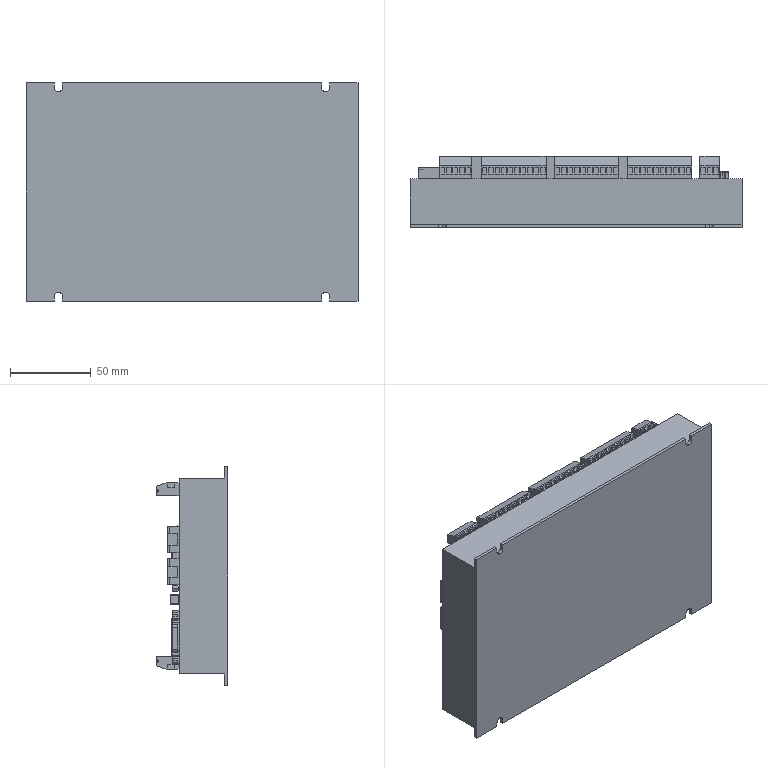Part | SolidWorks | features BaseBody 96 | 96 solids | 3160 faces | volume 778602 mm3 | plane 2120 | cylinder 620 | spline 388 | torus 24 | sphere 8 | commonest cylinder face diameters 1 x312 3 x128 4 x34 4.2 x30 4.8 x30 0.6 x28